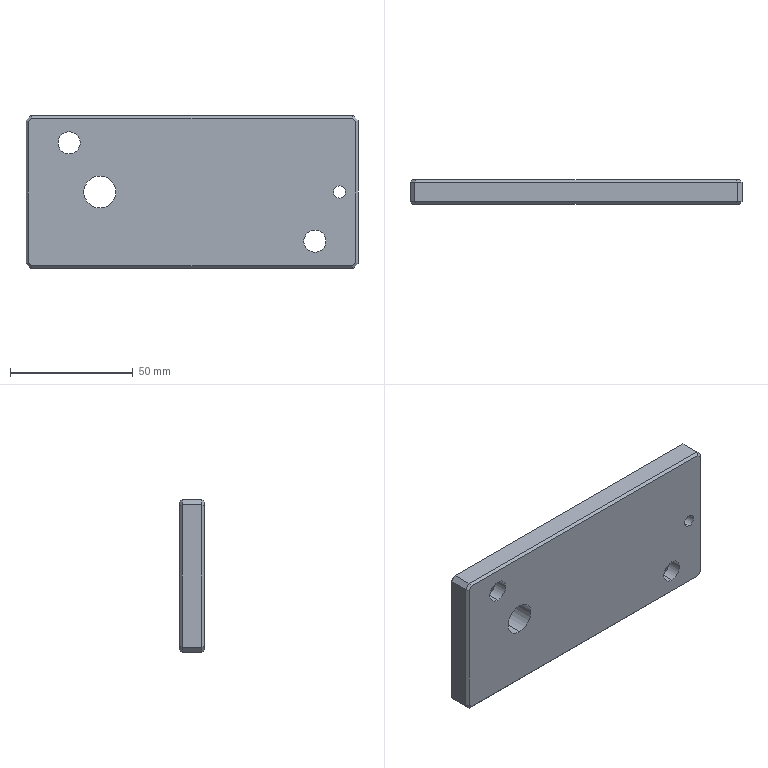Part | STEP file | Placa de deslize - Torre - 4-  1 cav | 1 solid | 38 faces | box 135 x 10 x 62 mm | volume 79689 mm3 | plane 26 | cylinder 8 | cone 4 | commonest cylinder face diameters 9 x4 5 x2 13 x2